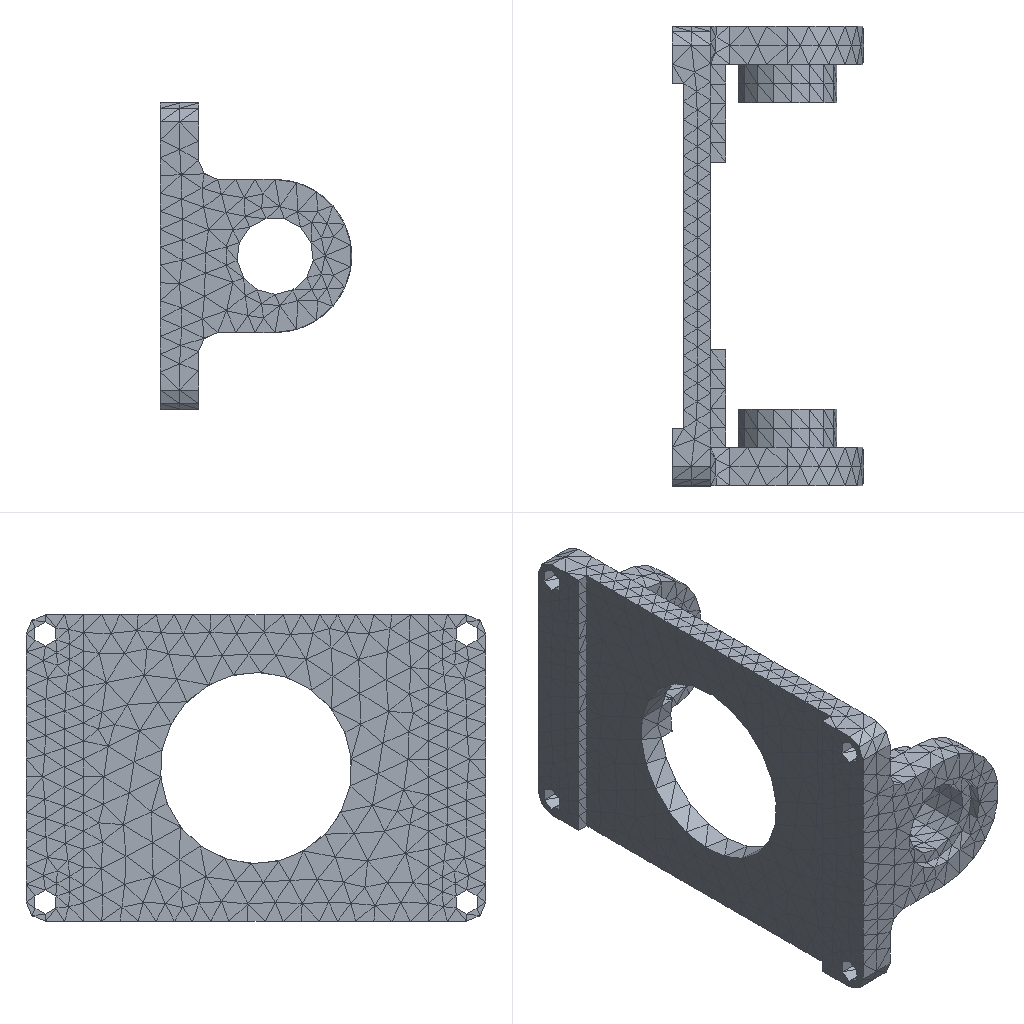Simulation study | nx simcenter
Set-up summary:
category,name,step,type,value,unit,region
solver,nx_nastran (Simcenter)
units,not stated in the deck,,not stated
analysis,deck,,static,static
analysis,solution,,SOL,101
load_step,SUBCASE 1,1,SUBCASE,SPC=1 LOAD=2
load_step,requested,,,1
mesh,nodes,,,7482
mesh,elements,,,3615
element_type,CTETRA,,solid,3615
load,nodal force total,,FX,-2000000.08,model units
load,nodal force total,,FY,0.0,model units
load,nodal force total,,FZ,0.0,model units
load,load commands in deck,,count,338
bc,support commands in deck,,count,582
analysis,NX solution 0,,Structural,Linear Statics - Single Constraint
check,setup vs results,,match,every grid point's frame and coordinates and every element id; grid points of CTETRA elements
Nastran input file, long lists of numbers shortened:
$*$$$$$$$$$$$$$$$$$$$$$$$$$$$$$$$$$$$$$$$$$$$$$$$$$$$$$$$$$$$$$$$$$
$*
$*                    NX v10.0.0.24 TRANSLATOR
$*                    FOR NX NASTRAN VERSION 10.0
$ (33 more lines like these left out)
ASSIGN OUTPUT2='105_sim1-solution_1.op2' UNIT=12
$*
$*$$$$$$$$$$$$$$$$$$$$$$$$$$$$$$$$$$$
$*
$* EXECUTIVE CONTROL
$*
$*$$$$$$$$$$$$$$$$$$$$$$$$$$$$$$$$$$$
$*
ID,NASTRAN,105_sim1-solution_1
SOL 101
CEND
$*
$*$$$$$$$$$$$$$$$$$$$$$$$$$$$$$$$$$$$
$*
$* CASE CONTROL
$*
$*$$$$$$$$$$$$$$$$$$$$$$$$$$$$$$$$$$$
$*
TITLE = Solution 1
ECHO = NONE
SPC = 1
OUTPUT
BCRESULTS(TRACTION,FORCE,PLOT) = ALL
DISPLACEMENT(PLOT) = ALL
ESE(PLOT) = ALL
FORCE(PLOT,CORNER) = ALL
OLOAD(PLOT) = ALL
SPCFORCES(PLOT) = ALL
STRAIN(PLOT,FIBER,CORNER) = ALL
STRESS(PLOT,CORNER) = ALL
$*  NX Step: Subcase - Static Loads 1
SUBCASE 1
LABEL = Subcase - Static Loads 1
LOAD = 2
$*
$*$$$$$$$$$$$$$$$$$$$$$$$$$$$$$$$$$$$
$*
$* BULK DATA
$*
$*$$$$$$$$$$$$$$$$$$$$$$$$$$$$$$$$$$$
$*
BEGIN BULK
$*
$* PARAM CARDS
$*
PARAM      K6ROT100.0000
PARAM     OIBULK     YES
PARAM    OMACHPR     YES
PARAM       POST      -2
PARAM    POSTEXT     YES
PARAM    UNITSYS   MN-MM
$*
$* GRID CARDS
$*
GRID*               7398               00.0000000000E+00-6.000000000E+01+
*       3.5000000000E+01               0
GRID*               7399               00.0000000000E+00-6.000000000E+01+
*       -3.500000000E+01               0
$ (14960 more lines like these left out)
$*
$* ELEMENT CARDS
$*
$*  NX Mesh Collector: Solid(1)
$*  NX Mesh: 3d_mesh(1)
CTETRA         1       1       1    6125    6149    6150      64    2541+
+             65      66    2540    6155
CTETRA         2       1    6149    2488       1       2    2542      67+
+             65      68      69      70
$ (7226 more lines like these left out)
$*
$* PROPERTY CARDS
$*
$*  NX Property: PSOLID1
PSOLID         1       1       0                           SMECH
$*
$* MATERIAL CARDS
$*
$*  NX Material: 2A12
MAT1           17.3119+7        0.3300002.8000-62.1355-5
MATT1          1       1               2               3
TABLEM1        1                                                        +
+        20.00007.3119+7 21.11007.3119+7 23.89007.3119+7 37.78007.3119+7+
+        51.67007.3119+7 65.56007.2429+7 79.44007.2429+7 93.33007.1739+7+
+       107.22007.1049+7121.11007.0359+7135.00006.9670+7148.89006.8980+7+
+       162.78006.8290+7176.67006.6910+7190.56006.6221+7204.44006.4841+7+
+       218.33006.3461+7232.22006.1392+7246.11006.0012+7260.00005.8633+7+
+       273.89005.7253+7287.78005.5184+7301.67005.3804+7315.56005.1735+7+
+       329.44004.9665+7343.33004.7596+7357.22004.6216+7371.11004.4147+7+
+           ENDT
TABLEM1        2                                                        +
+        20.00000.330000 21.11000.330000    ENDT
TABLEM1        3                                                        +
+        20.00002.1600-5 93.33002.2500-5107.22002.2662-5121.11002.2824-5+
+       135.00002.2968-5148.89002.3130-5162.78002.3274-5176.67002.3418-5+
+       190.56002.3544-5204.44002.3688-5218.33002.3814-5232.22002.3958-5+
+       246.11002.4066-5260.00002.4192-5273.89002.4300-5287.78002.4408-5+
+       301.67002.4498-5315.56002.4606-5329.44002.4696-5343.33002.4786-5+
+       357.22002.4876-5371.11002.4984-5385.00002.5110-5398.89002.5254-5+
+       412.78002.5398-5426.67002.5560-5    ENDT
$*
$* LOAD AND CONSTRAINT CARDS
$*
$*  NX Load and Constraint: Fixed(1)
SPC            1    2483  123456  0.0000
SPC            1    2484  123456  0.0000
SPC            1    2485  123456  0.0000
SPC            1    2486  123456  0.0000
$ (578 more lines like these left out)
$*  NX Load and Constraint: Force(1)
FORCE          2    5523       0 6412.32-1.00000  0.0000  0.0000
FORCE          2    5524       0 6410.25-1.00000  0.0000  0.0000
FORCE          2    5525       0 6412.32-1.00000  0.0000  0.0000
FORCE          2    5526       0 6412.32-1.00000  0.0000  0.0000
$ (334 more lines like these left out)
ENDDATA 1bf31b81
Results summary:
result,analysis,,,static
result,last_loadstep,,,1
result,primary field,,,displacements
result,max displacement,,,0.02204,model units
result,reaction total,,FX,2000000.875,model units
result,reaction total,,FY,0.02747,model units
result,reaction total,,FZ,0.01681,model units
result,NX solution 0,,loadcases,1,mm